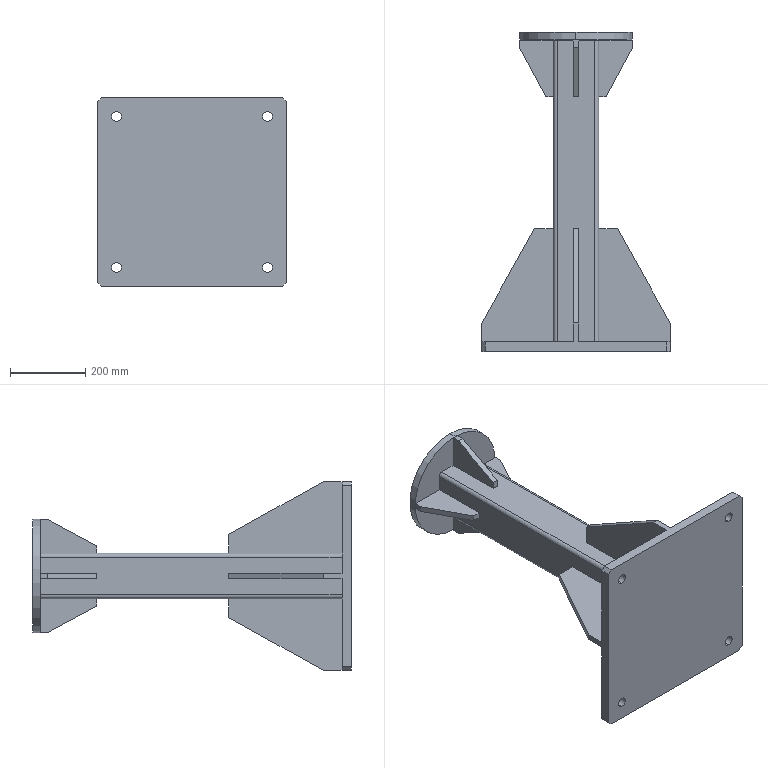Part | SolidWorks | features BaseBody 6, MoveFace 1 | 6 solids | 114 faces | box 500 x 845 x 500 mm | volume 14590958 mm3 | plane 70 | cylinder 34 | cone 10 | commonest cylinder face diameters 6.8 x8 8 x8 26 x8 10 x4 20 x4 300 x2